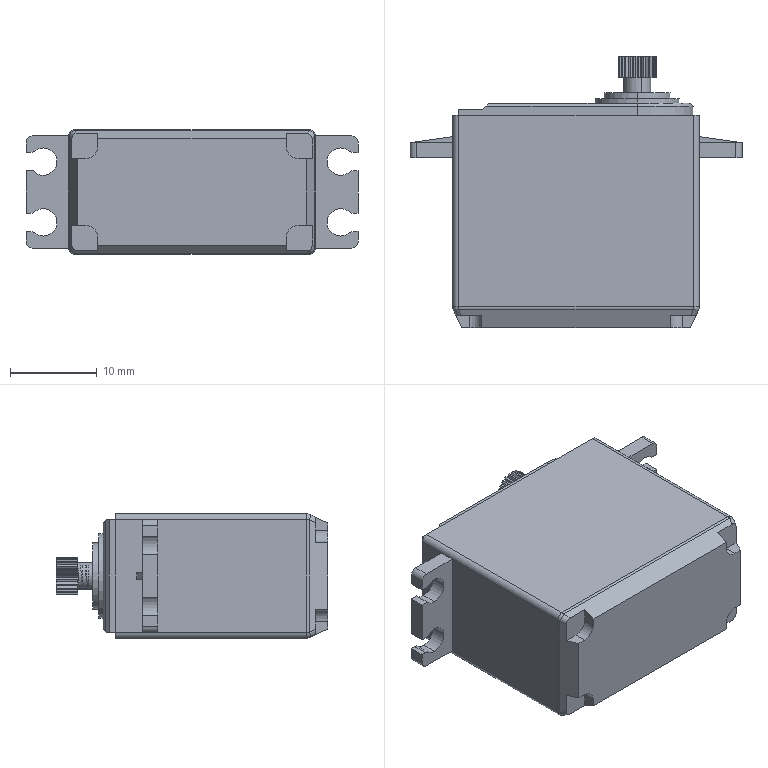Part | SolidWorks | 2 solids | 220 faces | box 38.29 x 31.325 x 14.35 mm | volume 10527 mm3 | plane 116 | cylinder 90 | spline 9 | sphere 4 | cone 1 | commonest cylinder face diameters 1.4 x24 4.361 x23 2.86 x18 3.15 x12 2.8 x4 3.1 x4